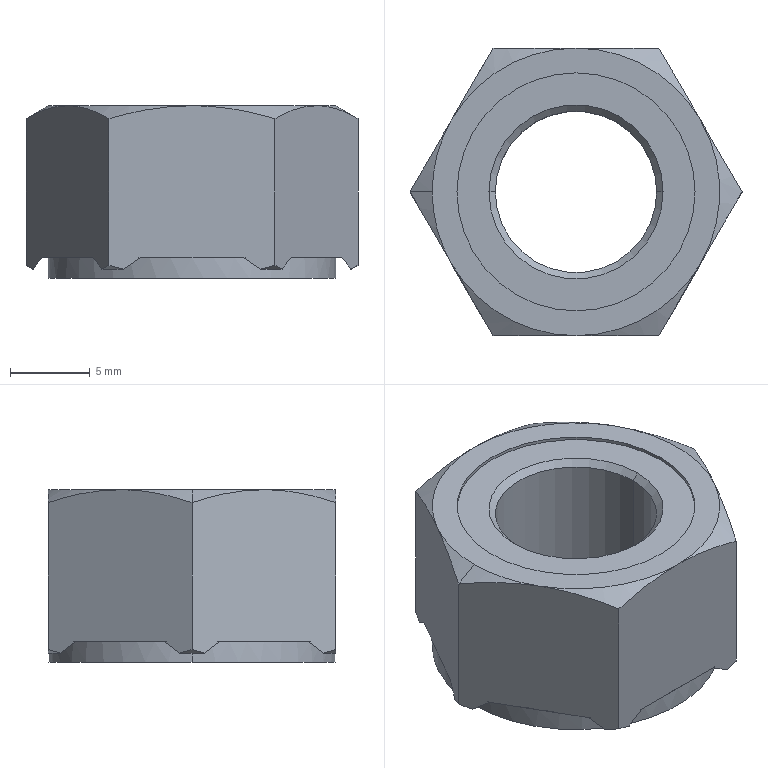Part | STEP file | M12_GB13681_2_VD-SYL0380DJ1006_ | 1 solid | 46 faces | box 20.785 x 18 x 10.8 mm | volume 2100 mm3 | cone 25 | plane 15 | cylinder 6 | commonest cylinder face diameters 10.106 x2 14.9 x2 18 x2